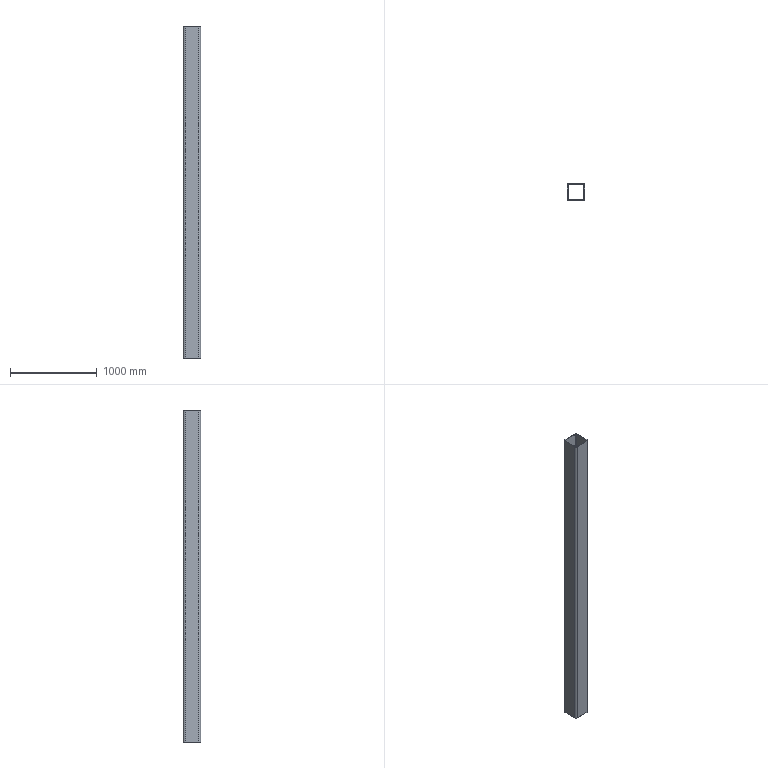Part | SolidWorks | features Extrusion 1 | 1 solid | 18 faces | box 200 x 200 x 3830 mm | volume 22689869 mm3 | plane 10 | cylinder 8 | commonest cylinder face diameters 24 x4 40 x4
STEP:
#1=CARTESIAN_POINT('',(-100.,-80.,3830.));
#2=VERTEX_POINT('',#1);
#3=CARTESIAN_POINT('',(-80.,-100.,3830.));
#4=VERTEX_POINT('',#3);
#5=CARTESIAN_POINT('',(-80.,-80.,3830.));
#6=DIRECTION('',(0.,0.,1.));
#7=DIRECTION('',(1.,0.,0.));
#8=AXIS2_PLACEMENT_3D('',#5,#6,#7);
#9=CIRCLE('',#8,20.);
#10=EDGE_CURVE('',#2,#4,#9,.T.);
#11=ORIENTED_EDGE('',*,*,#10,.T.);
#12=CARTESIAN_POINT('',(80.,-100.,3830.));
#13=VERTEX_POINT('',#12);
#14=CARTESIAN_POINT('',(-80.,-100.,3830.));
#15=DIRECTION('',(1.,0.,0.));
#16=VECTOR('',#15,1000.);
#17=LINE('',#14,#16);
#18=EDGE_CURVE('',#4,#13,#17,.T.);
#19=ORIENTED_EDGE('',*,*,#18,.T.);
#20=CARTESIAN_POINT('',(100.,-80.,3830.));
#21=VERTEX_POINT('',#20);
#22=CARTESIAN_POINT('',(80.,-80.,3830.));
#23=DIRECTION('',(0.,0.,1.));
#24=DIRECTION('',(1.,0.,0.));
#25=AXIS2_PLACEMENT_3D('',#22,#23,#24);
#26=CIRCLE('',#25,20.);
#27=EDGE_CURVE('',#13,#21,#26,.T.);
#28=ORIENTED_EDGE('',*,*,#27,.T.);
#29=CARTESIAN_POINT('',(100.,80.,3830.));
#30=VERTEX_POINT('',#29);
#31=CARTESIAN_POINT('',(100.,80.,3830.));
#32=DIRECTION('',(0.,1.,0.));
#33=VECTOR('',#32,1000.);
#34=LINE('',#31,#33);
#35=EDGE_CURVE('',#21,#30,#34,.T.);
#36=ORIENTED_EDGE('',*,*,#35,.T.);
#37=CARTESIAN_POINT('',(80.,100.,3830.));
#38=VERTEX_POINT('',#37);
#39=CARTESIAN_POINT('',(80.,80.,3830.));
#40=DIRECTION('',(0.,0.,1.));
#41=DIRECTION('',(-1.,0.,0.));
#42=AXIS2_PLACEMENT_3D('',#39,#40,#41);
#43=CIRCLE('',#42,20.);
#44=EDGE_CURVE('',#30,#38,#43,.T.);
#45=ORIENTED_EDGE('',*,*,#44,.T.);
#46=CARTESIAN_POINT('',(-80.,100.,3830.));
#47=VERTEX_POINT('',#46);
#48=CARTESIAN_POINT('',(-80.,100.,3830.));
#49=DIRECTION('',(-1.,0.,0.));
#50=VECTOR('',#49,1000.);
#51=LINE('',#48,#50);
#52=EDGE_CURVE('',#38,#47,#51,.T.);
#53=ORIENTED_EDGE('',*,*,#52,.T.);
#54=CARTESIAN_POINT('',(-100.,80.,3830.));
#55=VERTEX_POINT('',#54);
#56=CARTESIAN_POINT('',(-80.,80.,3830.));
#57=DIRECTION('',(0.,0.,1.));
#58=DIRECTION('',(1.,0.,0.));
#59=AXIS2_PLACEMENT_3D('',#56,#57,#58);
#60=CIRCLE('',#59,20.);
#61=EDGE_CURVE('',#47,#55,#60,.T.);
#62=ORIENTED_EDGE('',*,*,#61,.T.);
#63=CARTESIAN_POINT('',(-100.,80.,3830.));
#64=DIRECTION('',(0.,-1.,0.));
#65=VECTOR('',#64,1000.);
#66=LINE('',#63,#65);
#67=EDGE_CURVE('',#55,#2,#66,.T.);
#68=ORIENTED_EDGE('',*,*,#67,.T.);
#69=EDGE_LOOP('',(#11,#19,#28,#36,#45,#53,#62,#68));
#70=FACE_OUTER_BOUND('',#69,.T.);
#71=CARTESIAN_POINT('',(-92.,80.,3830.));
#72=VERTEX_POINT('',#71);
#73=CARTESIAN_POINT('',(-92.,-80.,3830.));
#74=VERTEX_POINT('',#73);
#75=CARTESIAN_POINT('',(-92.,80.,3830.));
#76=DIRECTION('',(0.,-1.,0.));
#77=VECTOR('',#76,1000.);
#78=LINE('',#75,#77);
#79=EDGE_CURVE('',#72,#74,#78,.T.);
#80=ORIENTED_EDGE('',*,*,#79,.F.);
#81=CARTESIAN_POINT('',(-80.,92.,3830.));
#82=VERTEX_POINT('',#81);
#83=CARTESIAN_POINT('',(-80.,80.,3830.));
#84=DIRECTION('',(0.,0.,1.));
#85=DIRECTION('',(1.,0.,0.));
#86=AXIS2_PLACEMENT_3D('',#83,#84,#85);
#87=CIRCLE('',#86,12.);
#88=EDGE_CURVE('',#82,#72,#87,.T.);
#89=ORIENTED_EDGE('',*,*,#88,.F.);
#90=CARTESIAN_POINT('',(80.,92.,3830.));
#91=VERTEX_POINT('',#90);
#92=CARTESIAN_POINT('',(-80.,92.,3830.));
#93=DIRECTION('',(-1.,0.,0.));
#94=VECTOR('',#93,1000.);
#95=LINE('',#92,#94);
#96=EDGE_CURVE('',#91,#82,#95,.T.);
#97=ORIENTED_EDGE('',*,*,#96,.F.);
#98=CARTESIAN_POINT('',(92.,80.,3830.));
#99=VERTEX_POINT('',#98);
#100=CARTESIAN_POINT('',(80.,80.,3830.));
#101=DIRECTION('',(0.,0.,1.));
#102=DIRECTION('',(-1.,0.,0.));
#103=AXIS2_PLACEMENT_3D('',#100,#101,#102);
#104=CIRCLE('',#103,12.);
#105=EDGE_CURVE('',#99,#91,#104,.T.);
#106=ORIENTED_EDGE('',*,*,#105,.F.);
#107=CARTESIAN_POINT('',(92.,-80.,3830.));
#108=VERTEX_POINT('',#107);
#109=CARTESIAN_POINT('',(92.,80.,3830.));
#110=DIRECTION('',(0.,1.,0.));
#111=VECTOR('',#110,1000.);
#112=LINE('',#109,#111);
#113=EDGE_CURVE('',#108,#99,#112,.T.);
#114=ORIENTED_EDGE('',*,*,#113,.F.);
#115=CARTESIAN_POINT('',(80.,-92.,3830.));
#116=VERTEX_POINT('',#115);
#117=CARTESIAN_POINT('',(80.,-80.,3830.));
#118=DIRECTION('',(0.,0.,1.));
#119=DIRECTION('',(1.,0.,0.));
#120=AXIS2_PLACEMENT_3D('',#117,#118,#119);
#121=CIRCLE('',#120,12.);
#122=EDGE_CURVE('',#116,#108,#121,.T.);
#123=ORIENTED_EDGE('',*,*,#122,.F.);
#124=CARTESIAN_POINT('',(-80.,-92.,3830.));
#125=VERTEX_POINT('',#124);
#126=CARTESIAN_POINT('',(-80.,-92.,3830.));
#127=DIRECTION('',(1.,0.,0.));
#128=VECTOR('',#127,1000.);
#129=LINE('',#126,#128);
#130=EDGE_CURVE('',#125,#116,#129,.T.);
#131=ORIENTED_EDGE('',*,*,#130,.F.);
#132=CARTESIAN_POINT('',(-80.,-80.,3830.));
#133=DIRECTION('',(0.,0.,1.));
#134=DIRECTION('',(1.,0.,0.));
#135=AXIS2_PLACEMENT_3D('',#132,#133,#134);
#136=CIRCLE('',#135,12.);
#137=EDGE_CURVE('',#74,#125,#136,.T.);
#138=ORIENTED_EDGE('',*,*,#137,.F.);
#139=EDGE_LOOP('',(#80,#89,#97,#106,#114,#123,#131,#138));
#140=FACE_BOUND('',#139,.T.);
#141=CARTESIAN_POINT('',(-80.,-80.,3830.));
#142=DIRECTION('',(0.,0.,1.));
#143=DIRECTION('',(1.,0.,0.));
#144=AXIS2_PLACEMENT_3D('',#141,#142,#143);
#145=PLANE('',#144);
#146=ADVANCED_FACE('',(#70,#140),#145,.T.);
#147=CARTESIAN_POINT('',(-100.,-80.,0.));
#148=VERTEX_POINT('',#147);
#149=CARTESIAN_POINT('',(-80.,-100.,0.));
#150=VERTEX_POINT('',#149);
#151=CARTESIAN_POINT('',(-80.,-80.,0.));
#152=DIRECTION('',(0.,0.,1.));
#153=DIRECTION('',(1.,0.,0.));
#154=AXIS2_PLACEMENT_3D('',#151,#152,#153);
#155=CIRCLE('',#154,20.);
#156=EDGE_CURVE('',#148,#150,#155,.T.);
#157=ORIENTED_EDGE('',*,*,#156,.F.);
#158=CARTESIAN_POINT('',(-100.,80.,0.));
#159=VERTEX_POINT('',#158);
#160=CARTESIAN_POINT('',(-100.,80.,0.));
#161=DIRECTION('',(0.,-1.,0.));
#162=VECTOR('',#161,1000.);
#163=LINE('',#160,#162);
#164=EDGE_CURVE('',#159,#148,#163,.T.);
#165=ORIENTED_EDGE('',*,*,#164,.F.);
#166=CARTESIAN_POINT('',(-80.,100.,0.));
#167=VERTEX_POINT('',#166);
#168=CARTESIAN_POINT('',(-80.,80.,0.));
#169=DIRECTION('',(0.,0.,1.));
#170=DIRECTION('',(1.,0.,0.));
#171=AXIS2_PLACEMENT_3D('',#168,#169,#170);
#172=CIRCLE('',#171,20.);
#173=EDGE_CURVE('',#167,#159,#172,.T.);
#174=ORIENTED_EDGE('',*,*,#173,.F.);
#175=CARTESIAN_POINT('',(80.,100.,0.));
#176=VERTEX_POINT('',#175);
#177=CARTESIAN_POINT('',(-80.,100.,0.));
#178=DIRECTION('',(-1.,0.,0.));
#179=VECTOR('',#178,1000.);
#180=LINE('',#177,#179);
#181=EDGE_CURVE('',#176,#167,#180,.T.);
#182=ORIENTED_EDGE('',*,*,#181,.F.);
#183=CARTESIAN_POINT('',(100.,80.,0.));
#184=VERTEX_POINT('',#183);
#185=CARTESIAN_POINT('',(80.,80.,0.));
#186=DIRECTION('',(0.,0.,1.));
#187=DIRECTION('',(-1.,0.,0.));
#188=AXIS2_PLACEMENT_3D('',#185,#186,#187);
#189=CIRCLE('',#188,20.);
#190=EDGE_CURVE('',#184,#176,#189,.T.);
#191=ORIENTED_EDGE('',*,*,#190,.F.);
#192=CARTESIAN_POINT('',(100.,-80.,0.));
#193=VERTEX_POINT('',#192);
#194=CARTESIAN_POINT('',(100.,80.,0.));
#195=DIRECTION('',(0.,1.,0.));
#196=VECTOR('',#195,1000.);
#197=LINE('',#194,#196);
#198=EDGE_CURVE('',#193,#184,#197,.T.);
#199=ORIENTED_EDGE('',*,*,#198,.F.);
#200=CARTESIAN_POINT('',(80.,-100.,0.));
#201=VERTEX_POINT('',#200);
#202=CARTESIAN_POINT('',(80.,-80.,0.));
#203=DIRECTION('',(0.,0.,1.));
#204=DIRECTION('',(1.,0.,0.));
#205=AXIS2_PLACEMENT_3D('',#202,#203,#204);
#206=CIRCLE('',#205,20.);
#207=EDGE_CURVE('',#201,#193,#206,.T.);
#208=ORIENTED_EDGE('',*,*,#207,.F.);
#209=CARTESIAN_POINT('',(-80.,-100.,0.));
#210=DIRECTION('',(1.,0.,0.));
#211=VECTOR('',#210,1000.);
#212=LINE('',#209,#211);
#213=EDGE_CURVE('',#150,#201,#212,.T.);
#214=ORIENTED_EDGE('',*,*,#213,.F.);
#215=EDGE_LOOP('',(#157,#165,#174,#182,#191,#199,#208,#214));
#216=FACE_OUTER_BOUND('',#215,.T.);
#217=CARTESIAN_POINT('',(-80.,92.,0.));
#218=VERTEX_POINT('',#217);
#219=CARTESIAN_POINT('',(-92.,80.,0.));
#220=VERTEX_POINT('',#219);
#221=CARTESIAN_POINT('',(-80.,80.,0.));
#222=DIRECTION('',(0.,0.,1.));
#223=DIRECTION('',(1.,0.,0.));
#224=AXIS2_PLACEMENT_3D('',#221,#222,#223);
#225=CIRCLE('',#224,12.);
#226=EDGE_CURVE('',#218,#220,#225,.T.);
#227=ORIENTED_EDGE('',*,*,#226,.T.);
#228=CARTESIAN_POINT('',(-92.,-80.,0.));
#229=VERTEX_POINT('',#228);
#230=CARTESIAN_POINT('',(-92.,80.,0.));
#231=DIRECTION('',(0.,-1.,0.));
#232=VECTOR('',#231,1000.);
#233=LINE('',#230,#232);
#234=EDGE_CURVE('',#220,#229,#233,.T.);
#235=ORIENTED_EDGE('',*,*,#234,.T.);
#236=CARTESIAN_POINT('',(-80.,-92.,0.));
#237=VERTEX_POINT('',#236);
#238=CARTESIAN_POINT('',(-80.,-80.,0.));
#239=DIRECTION('',(0.,0.,1.));
#240=DIRECTION('',(1.,0.,0.));
#241=AXIS2_PLACEMENT_3D('',#238,#239,#240);
#242=CIRCLE('',#241,12.);
#243=EDGE_CURVE('',#229,#237,#242,.T.);
#244=ORIENTED_EDGE('',*,*,#243,.T.);
#245=CARTESIAN_POINT('',(80.,-92.,0.));
#246=VERTEX_POINT('',#245);
#247=CARTESIAN_POINT('',(-80.,-92.,0.));
#248=DIRECTION('',(1.,0.,0.));
#249=VECTOR('',#248,1000.);
#250=LINE('',#247,#249);
#251=EDGE_CURVE('',#237,#246,#250,.T.);
#252=ORIENTED_EDGE('',*,*,#251,.T.);
#253=CARTESIAN_POINT('',(92.,-80.,0.));
#254=VERTEX_POINT('',#253);
#255=CARTESIAN_POINT('',(80.,-80.,0.));
#256=DIRECTION('',(0.,0.,1.));
#257=DIRECTION('',(1.,0.,0.));
#258=AXIS2_PLACEMENT_3D('',#255,#256,#257);
#259=CIRCLE('',#258,12.);
#260=EDGE_CURVE('',#246,#254,#259,.T.);
#261=ORIENTED_EDGE('',*,*,#260,.T.);
#262=CARTESIAN_POINT('',(92.,80.,0.));
#263=VERTEX_POINT('',#262);
#264=CARTESIAN_POINT('',(92.,80.,0.));
#265=DIRECTION('',(0.,1.,0.));
#266=VECTOR('',#265,1000.);
#267=LINE('',#264,#266);
#268=EDGE_CURVE('',#254,#263,#267,.T.);
#269=ORIENTED_EDGE('',*,*,#268,.T.);
#270=CARTESIAN_POINT('',(80.,92.,0.));
#271=VERTEX_POINT('',#270);
#272=CARTESIAN_POINT('',(80.,80.,0.));
#273=DIRECTION('',(0.,0.,1.));
#274=DIRECTION('',(-1.,0.,0.));
#275=AXIS2_PLACEMENT_3D('',#272,#273,#274);
#276=CIRCLE('',#275,12.);
#277=EDGE_CURVE('',#263,#271,#276,.T.);
#278=ORIENTED_EDGE('',*,*,#277,.T.);
#279=CARTESIAN_POINT('',(-80.,92.,0.));
#280=DIRECTION('',(-1.,0.,0.));
#281=VECTOR('',#280,1000.);
#282=LINE('',#279,#281);
#283=EDGE_CURVE('',#271,#218,#282,.T.);
#284=ORIENTED_EDGE('',*,*,#283,.T.);
#285=EDGE_LOOP('',(#227,#235,#244,#252,#261,#269,#278,#284));
#286=FACE_BOUND('',#285,.T.);
#287=CARTESIAN_POINT('',(-80.,-80.,0.));
#288=DIRECTION('',(0.,0.,1.));
#289=DIRECTION('',(1.,0.,0.));
#290=AXIS2_PLACEMENT_3D('',#287,#288,#289);
#291=PLANE('',#290);
#292=ADVANCED_FACE('',(#216,#286),#291,.F.);
#293=ORIENTED_EDGE('',*,*,#156,.T.);
#294=CARTESIAN_POINT('',(-80.,-100.,3830.));
#295=DIRECTION('',(0.,0.,-1.));
#296=VECTOR('',#295,1000.);
#297=LINE('',#294,#296);
#298=EDGE_CURVE('',#4,#150,#297,.T.);
#299=ORIENTED_EDGE('',*,*,#298,.F.);
#300=ORIENTED_EDGE('',*,*,#10,.F.);
#301=CARTESIAN_POINT('',(-100.,-80.,3830.));
#302=DIRECTION('',(0.,0.,-1.));
#303=VECTOR('',#302,1000.);
#304=LINE('',#301,#303);
#305=EDGE_CURVE('',#2,#148,#304,.T.);
#306=ORIENTED_EDGE('',*,*,#305,.T.);
#307=EDGE_LOOP('',(#293,#299,#300,#306));
#308=FACE_OUTER_BOUND('',#307,.T.);
#309=CARTESIAN_POINT('',(-80.,-80.,3830.));
#310=DIRECTION('',(0.,0.,-1.));
#311=DIRECTION('',(-1.,0.,0.));
#312=AXIS2_PLACEMENT_3D('',#309,#310,#311);
#313=CYLINDRICAL_SURFACE('',#312,20.);
#314=ADVANCED_FACE('',(#308),#313,.T.);
#315=ORIENTED_EDGE('',*,*,#213,.T.);
#316=CARTESIAN_POINT('',(80.,-100.,3830.));
#317=DIRECTION('',(0.,0.,-1.));
#318=VECTOR('',#317,1000.);
#319=LINE('',#316,#318);
#320=EDGE_CURVE('',#13,#201,#319,.T.);
#321=ORIENTED_EDGE('',*,*,#320,.F.);
#322=ORIENTED_EDGE('',*,*,#18,.F.);
#323=ORIENTED_EDGE('',*,*,#298,.T.);
#324=EDGE_LOOP('',(#315,#321,#322,#323));
#325=FACE_OUTER_BOUND('',#324,.T.);
#326=CARTESIAN_POINT('',(-80.,-100.,3830.));
#327=DIRECTION('',(0.,1.,0.));
#328=DIRECTION('',(0.,0.,1.));
#329=AXIS2_PLACEMENT_3D('',#326,#327,#328);
#330=PLANE('',#329);
#331=ADVANCED_FACE('',(#325),#330,.F.);
#332=ORIENTED_EDGE('',*,*,#207,.T.);
#333=CARTESIAN_POINT('',(100.,-80.,3830.));
#334=DIRECTION('',(0.,0.,-1.));
#335=VECTOR('',#334,1000.);
#336=LINE('',#333,#335);
#337=EDGE_CURVE('',#21,#193,#336,.T.);
#338=ORIENTED_EDGE('',*,*,#337,.F.);
#339=ORIENTED_EDGE('',*,*,#27,.F.);
#340=ORIENTED_EDGE('',*,*,#320,.T.);
#341=EDGE_LOOP('',(#332,#338,#339,#340));
#342=FACE_OUTER_BOUND('',#341,.T.);
#343=CARTESIAN_POINT('',(80.,-80.,3830.));
#344=DIRECTION('',(0.,0.,-1.));
#345=DIRECTION('',(-1.,0.,0.));
#346=AXIS2_PLACEMENT_3D('',#343,#344,#345);
#347=CYLINDRICAL_SURFACE('',#346,20.);
#348=ADVANCED_FACE('',(#342),#347,.T.);
#349=ORIENTED_EDGE('',*,*,#198,.T.);
#350=CARTESIAN_POINT('',(100.,80.,3830.));
#351=DIRECTION('',(0.,0.,-1.));
#352=VECTOR('',#351,1000.);
#353=LINE('',#350,#352);
#354=EDGE_CURVE('',#30,#184,#353,.T.);
#355=ORIENTED_EDGE('',*,*,#354,.F.);
#356=ORIENTED_EDGE('',*,*,#35,.F.);
#357=ORIENTED_EDGE('',*,*,#337,.T.);
#358=EDGE_LOOP('',(#349,#355,#356,#357));
#359=FACE_OUTER_BOUND('',#358,.T.);
#360=CARTESIAN_POINT('',(100.,80.,3830.));
#361=DIRECTION('',(-1.,0.,0.));
#362=DIRECTION('',(0.,-1.,0.));
#363=AXIS2_PLACEMENT_3D('',#360,#361,#362);
#364=PLANE('',#363);
#365=ADVANCED_FACE('',(#359),#364,.F.);
#366=ORIENTED_EDGE('',*,*,#190,.T.);
#367=CARTESIAN_POINT('',(80.,100.,3830.));
#368=DIRECTION('',(0.,0.,-1.));
#369=VECTOR('',#368,1000.);
#370=LINE('',#367,#369);
#371=EDGE_CURVE('',#38,#176,#370,.T.);
#372=ORIENTED_EDGE('',*,*,#371,.F.);
#373=ORIENTED_EDGE('',*,*,#44,.F.);
#374=ORIENTED_EDGE('',*,*,#354,.T.);
#375=EDGE_LOOP('',(#366,#372,#373,#374));
#376=FACE_OUTER_BOUND('',#375,.T.);
#377=CARTESIAN_POINT('',(80.,80.,3830.));
#378=DIRECTION('',(0.,0.,-1.));
#379=DIRECTION('',(-1.,0.,0.));
#380=AXIS2_PLACEMENT_3D('',#377,#378,#379);
#381=CYLINDRICAL_SURFACE('',#380,20.);
#382=ADVANCED_FACE('',(#376),#381,.T.);
#383=ORIENTED_EDGE('',*,*,#181,.T.);
#384=CARTESIAN_POINT('',(-80.,100.,3830.));
#385=DIRECTION('',(0.,0.,-1.));
#386=VECTOR('',#385,1000.);
#387=LINE('',#384,#386);
#388=EDGE_CURVE('',#47,#167,#387,.T.);
#389=ORIENTED_EDGE('',*,*,#388,.F.);
#390=ORIENTED_EDGE('',*,*,#52,.F.);
#391=ORIENTED_EDGE('',*,*,#371,.T.);
#392=EDGE_LOOP('',(#383,#389,#390,#391));
#393=FACE_OUTER_BOUND('',#392,.T.);
#394=CARTESIAN_POINT('',(-80.,100.,3830.));
#395=DIRECTION('',(0.,-1.,0.));
#396=DIRECTION('',(0.,0.,-1.));
#397=AXIS2_PLACEMENT_3D('',#394,#395,#396);
#398=PLANE('',#397);
#399=ADVANCED_FACE('',(#393),#398,.F.);
#400=ORIENTED_EDGE('',*,*,#173,.T.);
#401=CARTESIAN_POINT('',(-100.,80.,3830.));
#402=DIRECTION('',(0.,0.,-1.));
#403=VECTOR('',#402,1000.);
#404=LINE('',#401,#403);
#405=EDGE_CURVE('',#55,#159,#404,.T.);
#406=ORIENTED_EDGE('',*,*,#405,.F.);
#407=ORIENTED_EDGE('',*,*,#61,.F.);
#408=ORIENTED_EDGE('',*,*,#388,.T.);
#409=EDGE_LOOP('',(#400,#406,#407,#408));
#410=FACE_OUTER_BOUND('',#409,.T.);
#411=CARTESIAN_POINT('',(-80.,80.,3830.));
#412=DIRECTION('',(0.,0.,-1.));
#413=DIRECTION('',(-1.,0.,0.));
#414=AXIS2_PLACEMENT_3D('',#411,#412,#413);
#415=CYLINDRICAL_SURFACE('',#414,20.);
#416=ADVANCED_FACE('',(#410),#415,.T.);
#417=ORIENTED_EDGE('',*,*,#164,.T.);
#418=ORIENTED_EDGE('',*,*,#305,.F.);
#419=ORIENTED_EDGE('',*,*,#67,.F.);
#420=ORIENTED_EDGE('',*,*,#405,.T.);
#421=EDGE_LOOP('',(#417,#418,#419,#420));
#422=FACE_OUTER_BOUND('',#421,.T.);
#423=CARTESIAN_POINT('',(-100.,80.,3830.));
#424=DIRECTION('',(1.,0.,0.));
#425=DIRECTION('',(0.,1.,0.));
#426=AXIS2_PLACEMENT_3D('',#423,#424,#425);
#427=PLANE('',#426);
#428=ADVANCED_FACE('',(#422),#427,.F.);
#429=ORIENTED_EDGE('',*,*,#226,.F.);
#430=CARTESIAN_POINT('',(-80.,92.,3830.));
#431=DIRECTION('',(0.,0.,-1.));
#432=VECTOR('',#431,1000.);
#433=LINE('',#430,#432);
#434=EDGE_CURVE('',#82,#218,#433,.T.);
#435=ORIENTED_EDGE('',*,*,#434,.F.);
#436=ORIENTED_EDGE('',*,*,#88,.T.);
#437=CARTESIAN_POINT('',(-92.,80.,3830.));
#438=DIRECTION('',(0.,0.,-1.));
#439=VECTOR('',#438,1000.);
#440=LINE('',#437,#439);
#441=EDGE_CURVE('',#72,#220,#440,.T.);
#442=ORIENTED_EDGE('',*,*,#441,.T.);
#443=EDGE_LOOP('',(#429,#435,#436,#442));
#444=FACE_OUTER_BOUND('',#443,.T.);
#445=CARTESIAN_POINT('',(-80.,80.,3830.));
#446=DIRECTION('',(0.,0.,-1.));
#447=DIRECTION('',(-1.,0.,0.));
#448=AXIS2_PLACEMENT_3D('',#445,#446,#447);
#449=CYLINDRICAL_SURFACE('',#448,12.);
#450=ADVANCED_FACE('',(#444),#449,.F.);
#451=ORIENTED_EDGE('',*,*,#234,.F.);
#452=ORIENTED_EDGE('',*,*,#441,.F.);
#453=ORIENTED_EDGE('',*,*,#79,.T.);
#454=CARTESIAN_POINT('',(-92.,-80.,3830.));
#455=DIRECTION('',(0.,0.,-1.));
#456=VECTOR('',#455,1000.);
#457=LINE('',#454,#456);
#458=EDGE_CURVE('',#74,#229,#457,.T.);
#459=ORIENTED_EDGE('',*,*,#458,.T.);
#460=EDGE_LOOP('',(#451,#452,#453,#459));
#461=FACE_OUTER_BOUND('',#460,.T.);
#462=CARTESIAN_POINT('',(-92.,80.,3830.));
#463=DIRECTION('',(1.,0.,0.));
#464=DIRECTION('',(0.,0.,-1.));
#465=AXIS2_PLACEMENT_3D('',#462,#463,#464);
#466=PLANE('',#465);
#467=ADVANCED_FACE('',(#461),#466,.T.);
#468=ORIENTED_EDGE('',*,*,#243,.F.);
#469=ORIENTED_EDGE('',*,*,#458,.F.);
#470=ORIENTED_EDGE('',*,*,#137,.T.);
#471=CARTESIAN_POINT('',(-80.,-92.,3830.));
#472=DIRECTION('',(0.,0.,-1.));
#473=VECTOR('',#472,1000.);
#474=LINE('',#471,#473);
#475=EDGE_CURVE('',#125,#237,#474,.T.);
#476=ORIENTED_EDGE('',*,*,#475,.T.);
#477=EDGE_LOOP('',(#468,#469,#470,#476));
#478=FACE_OUTER_BOUND('',#477,.T.);
#479=CARTESIAN_POINT('',(-80.,-80.,3830.));
#480=DIRECTION('',(0.,0.,-1.));
#481=DIRECTION('',(-1.,0.,0.));
#482=AXIS2_PLACEMENT_3D('',#479,#480,#481);
#483=CYLINDRICAL_SURFACE('',#482,12.);
#484=ADVANCED_FACE('',(#478),#483,.F.);
#485=ORIENTED_EDGE('',*,*,#251,.F.);
#486=ORIENTED_EDGE('',*,*,#475,.F.);
#487=ORIENTED_EDGE('',*,*,#130,.T.);
#488=CARTESIAN_POINT('',(80.,-92.,3830.));
#489=DIRECTION('',(0.,0.,-1.));
#490=VECTOR('',#489,1000.);
#491=LINE('',#488,#490);
#492=EDGE_CURVE('',#116,#246,#491,.T.);
#493=ORIENTED_EDGE('',*,*,#492,.T.);
#494=EDGE_LOOP('',(#485,#486,#487,#493));
#495=FACE_OUTER_BOUND('',#494,.T.);
#496=CARTESIAN_POINT('',(-80.,-92.,3830.));
#497=DIRECTION('',(0.,1.,0.));
#498=DIRECTION('',(0.,0.,1.));
#499=AXIS2_PLACEMENT_3D('',#496,#497,#498);
#500=PLANE('',#499);
#501=ADVANCED_FACE('',(#495),#500,.T.);
#502=ORIENTED_EDGE('',*,*,#260,.F.);
#503=ORIENTED_EDGE('',*,*,#492,.F.);
#504=ORIENTED_EDGE('',*,*,#122,.T.);
#505=CARTESIAN_POINT('',(92.,-80.,3830.));
#506=DIRECTION('',(0.,0.,-1.));
#507=VECTOR('',#506,1000.);
#508=LINE('',#505,#507);
#509=EDGE_CURVE('',#108,#254,#508,.T.);
#510=ORIENTED_EDGE('',*,*,#509,.T.);
#511=EDGE_LOOP('',(#502,#503,#504,#510));
#512=FACE_OUTER_BOUND('',#511,.T.);
#513=CARTESIAN_POINT('',(80.,-80.,3830.));
#514=DIRECTION('',(0.,0.,-1.));
#515=DIRECTION('',(-1.,0.,0.));
#516=AXIS2_PLACEMENT_3D('',#513,#514,#515);
#517=CYLINDRICAL_SURFACE('',#516,12.);
#518=ADVANCED_FACE('',(#512),#517,.F.);
#519=ORIENTED_EDGE('',*,*,#268,.F.);
#520=ORIENTED_EDGE('',*,*,#509,.F.);
#521=ORIENTED_EDGE('',*,*,#113,.T.);
#522=CARTESIAN_POINT('',(92.,80.,3830.));
#523=DIRECTION('',(0.,0.,-1.));
#524=VECTOR('',#523,1000.);
#525=LINE('',#522,#524);
#526=EDGE_CURVE('',#99,#263,#525,.T.);
#527=ORIENTED_EDGE('',*,*,#526,.T.);
#528=EDGE_LOOP('',(#519,#520,#521,#527));
#529=FACE_OUTER_BOUND('',#528,.T.);
#530=CARTESIAN_POINT('',(92.,80.,3830.));
#531=DIRECTION('',(-1.,0.,0.));
#532=DIRECTION('',(0.,-1.,0.));
#533=AXIS2_PLACEMENT_3D('',#530,#531,#532);
#534=PLANE('',#533);
#535=ADVANCED_FACE('',(#529),#534,.T.);
#536=ORIENTED_EDGE('',*,*,#277,.F.);
#537=ORIENTED_EDGE('',*,*,#526,.F.);
#538=ORIENTED_EDGE('',*,*,#105,.T.);
#539=CARTESIAN_POINT('',(80.,92.,3830.));
#540=DIRECTION('',(0.,0.,-1.));
#541=VECTOR('',#540,1000.);
#542=LINE('',#539,#541);
#543=EDGE_CURVE('',#91,#271,#542,.T.);
#544=ORIENTED_EDGE('',*,*,#543,.T.);
#545=EDGE_LOOP('',(#536,#537,#538,#544));
#546=FACE_OUTER_BOUND('',#545,.T.);
#547=CARTESIAN_POINT('',(80.,80.,3830.));
#548=DIRECTION('',(0.,0.,-1.));
#549=DIRECTION('',(-1.,0.,0.));
#550=AXIS2_PLACEMENT_3D('',#547,#548,#549);
#551=CYLINDRICAL_SURFACE('',#550,12.);
#552=ADVANCED_FACE('',(#546),#551,.F.);
#553=ORIENTED_EDGE('',*,*,#283,.F.);
#554=ORIENTED_EDGE('',*,*,#543,.F.);
#555=ORIENTED_EDGE('',*,*,#96,.T.);
#556=ORIENTED_EDGE('',*,*,#434,.T.);
#557=EDGE_LOOP('',(#553,#554,#555,#556));
#558=FACE_OUTER_BOUND('',#557,.T.);
#559=CARTESIAN_POINT('',(-80.,92.,3830.));
#560=DIRECTION('',(0.,-1.,0.));
#561=DIRECTION('',(0.,0.,-1.));
#562=AXIS2_PLACEMENT_3D('',#559,#560,#561);
#563=PLANE('',#562);
#564=ADVANCED_FACE('',(#558),#563,.T.);
#565=CLOSED_SHELL('',(#146,#292,#314,#331,#348,#365,#382,#399,#416,#428,#450,#467,#484,#501,#518,#535,#552,#564));
#566=MANIFOLD_SOLID_BREP('',#565);
#567=CARTESIAN_POINT('',(0.,0.,0.));
#568=DIRECTION('',(0.,0.,1.));
#569=DIRECTION('',(1.,0.,0.));
#570=AXIS2_PLACEMENT_3D('',#567,#568,#569);
#571=(LENGTH_UNIT()NAMED_UNIT(*)SI_UNIT(.MILLI.,.METRE.));
#572=UNCERTAINTY_MEASURE_WITH_UNIT(LENGTH_MEASURE(0.00001),#571,'','');
#573=(NAMED_UNIT(*)PLANE_ANGLE_UNIT()SI_UNIT($,.RADIAN.));
#574=(NAMED_UNIT(*)SI_UNIT($,.STERADIAN.)SOLID_ANGLE_UNIT());
#575=(GEOMETRIC_REPRESENTATION_CONTEXT(3)GLOBAL_UNCERTAINTY_ASSIGNED_CONTEXT((#572))GLOBAL_UNIT_ASSIGNED_CONTEXT((#571,#573,#574))REPRESENTATION_CONTEXT('',''));
#576=ADVANCED_BREP_SHAPE_REPRESENTATION('',(#566,#570),#575);